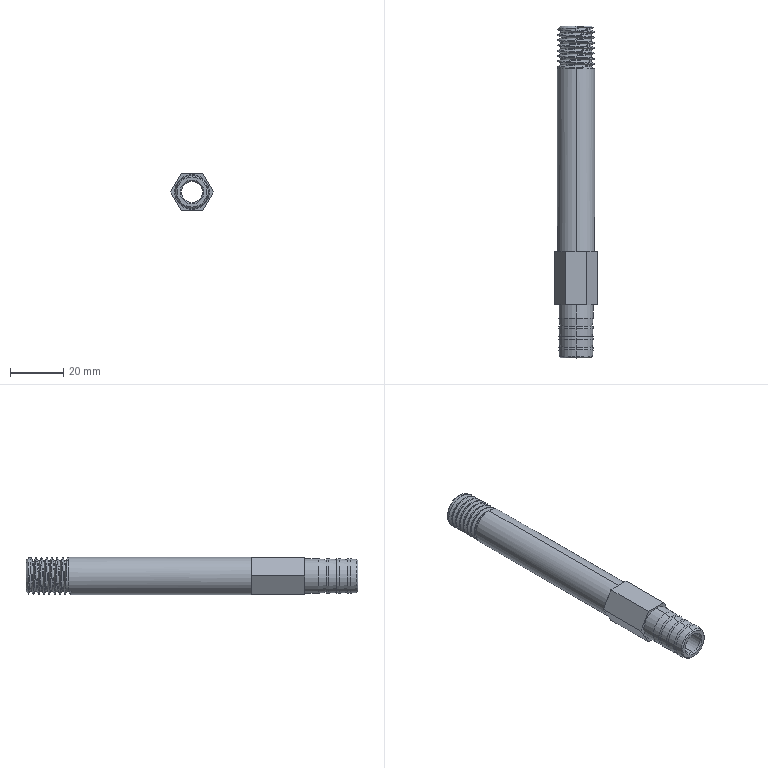Part | SolidWorks | features BaseBody 1 | 1 solid | 82 faces | box 16.166 x 125 x 14 mm | volume 12265 mm3 | cylinder 45 | plane 21 | cone 14 | spline 2 | commonest cylinder face diameters 13.6 x17 11.6 x16 13 x8 8 x2 14 x2